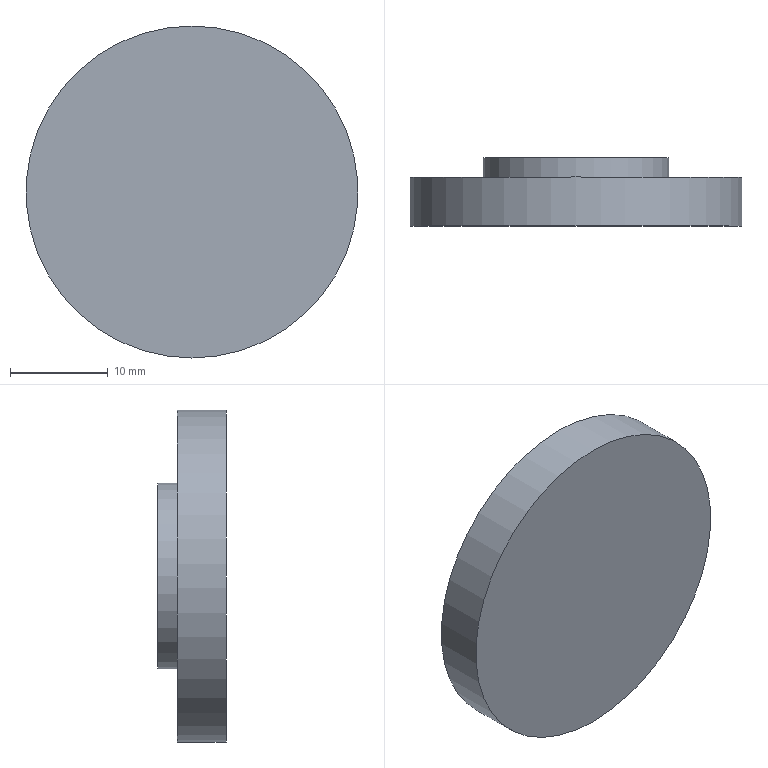Part | STEP file | zhoutao_φ16 | 1 solid | 7 faces | box 34 x 7 x 34 mm | volume 4705 mm3 | plane 4 | cylinder 3 | commonest cylinder face diameters 16 x1 19 x1 34 x1
STEP:
#1=CARTESIAN_POINT('',(0.,0.,0.));
#2=DIRECTION('',(0.,0.,1.));
#3=DIRECTION('',(1.,0.,0.));
#4=AXIS2_PLACEMENT_3D('',#1,#2,#3);
#5=CARTESIAN_POINT('',(0.,5.,17.));
#6=VERTEX_POINT('',#5);
#7=CARTESIAN_POINT('',(0.,5.,0.));
#8=DIRECTION('',(0.,1.,0.));
#9=DIRECTION('',(0.,0.,1.));
#10=AXIS2_PLACEMENT_3D('',#7,#8,#9);
#11=CIRCLE('',#10,17.);
#12=CARTESIAN_POINT('',(0.,5.,0.));
#13=DIRECTION('',(0.,-1.,0.));
#14=DIRECTION('',(0.,0.,-1.));
#15=AXIS2_PLACEMENT_3D('',#12,#13,#14);
#16=CYLINDRICAL_SURFACE('',#15,17.);
#17=CARTESIAN_POINT('',(9.425,0.));
#18=DIRECTION('',(-1.,0.));
#19=VECTOR('',#18,1.);
#20=LINE('',#17,#19);
#21=(GEOMETRIC_REPRESENTATION_CONTEXT(2)PARAMETRIC_REPRESENTATION_CONTEXT()REPRESENTATION_CONTEXT('',''));
#22=DEFINITIONAL_REPRESENTATION('',(#20),#21);
#23=PCURVE('',#16,#22);
#24=CARTESIAN_POINT('',(0.,5.,0.));
#25=DIRECTION('',(0.,1.,0.));
#26=DIRECTION('',(0.,0.,1.));
#27=AXIS2_PLACEMENT_3D('',#24,#25,#26);
#28=PLANE('',#27);
#29=CARTESIAN_POINT('',(0.,0.));
#30=DIRECTION('',(1.,0.));
#31=AXIS2_PLACEMENT_2D('',#29,#30);
#32=CIRCLE('',#31,17.);
#33=(GEOMETRIC_REPRESENTATION_CONTEXT(2)PARAMETRIC_REPRESENTATION_CONTEXT()REPRESENTATION_CONTEXT('',''));
#34=DEFINITIONAL_REPRESENTATION('',(#32),#33);
#35=PCURVE('',#28,#34);
#36=SURFACE_CURVE('',#11,(#23,#35),.PCURVE_S1.);
#37=EDGE_CURVE('',#6,#6,#36,.T.);
#38=ORIENTED_EDGE('',*,*,#37,.F.);
#39=CARTESIAN_POINT('',(0.,0.,17.));
#40=VERTEX_POINT('',#39);
#41=CARTESIAN_POINT('',(0.,5.,17.));
#42=CARTESIAN_POINT('',(0.,0.,17.));
#43=B_SPLINE_CURVE_WITH_KNOTS('',1,(#41,#42),.UNSPECIFIED.,.F.,.F.,(2,2),(0.,5.),.PIECEWISE_BEZIER_KNOTS.);
#44=CARTESIAN_POINT('',(9.425,0.));
#45=DIRECTION('',(0.,1.));
#46=VECTOR('',#45,1.);
#47=LINE('',#44,#46);
#48=(GEOMETRIC_REPRESENTATION_CONTEXT(2)PARAMETRIC_REPRESENTATION_CONTEXT()REPRESENTATION_CONTEXT('',''));
#49=DEFINITIONAL_REPRESENTATION('',(#47),#48);
#50=PCURVE('',#16,#49);
#51=CARTESIAN_POINT('',(3.142,0.));
#52=DIRECTION('',(0.,1.));
#53=VECTOR('',#52,1.);
#54=LINE('',#51,#53);
#55=(GEOMETRIC_REPRESENTATION_CONTEXT(2)PARAMETRIC_REPRESENTATION_CONTEXT()REPRESENTATION_CONTEXT('',''));
#56=DEFINITIONAL_REPRESENTATION('',(#54),#55);
#57=PCURVE('',#16,#56);
#58=SEAM_CURVE('',#43,(#50,#57),.PCURVE_S1.);
#59=EDGE_CURVE('',#6,#40,#58,.T.);
#60=ORIENTED_EDGE('',*,*,#59,.T.);
#61=CARTESIAN_POINT('',(0.,0.,0.));
#62=DIRECTION('',(0.,1.,0.));
#63=DIRECTION('',(0.,0.,1.));
#64=AXIS2_PLACEMENT_3D('',#61,#62,#63);
#65=CIRCLE('',#64,17.);
#66=CARTESIAN_POINT('',(9.425,5.));
#67=DIRECTION('',(-1.,0.));
#68=VECTOR('',#67,1.);
#69=LINE('',#66,#68);
#70=(GEOMETRIC_REPRESENTATION_CONTEXT(2)PARAMETRIC_REPRESENTATION_CONTEXT()REPRESENTATION_CONTEXT('',''));
#71=DEFINITIONAL_REPRESENTATION('',(#69),#70);
#72=PCURVE('',#16,#71);
#73=CARTESIAN_POINT('',(0.,0.,0.));
#74=DIRECTION('',(0.,1.,0.));
#75=DIRECTION('',(0.,0.,1.));
#76=AXIS2_PLACEMENT_3D('',#73,#74,#75);
#77=PLANE('',#76);
#78=CARTESIAN_POINT('',(0.,0.));
#79=DIRECTION('',(1.,0.));
#80=AXIS2_PLACEMENT_2D('',#78,#79);
#81=CIRCLE('',#80,17.);
#82=(GEOMETRIC_REPRESENTATION_CONTEXT(2)PARAMETRIC_REPRESENTATION_CONTEXT()REPRESENTATION_CONTEXT('',''));
#83=DEFINITIONAL_REPRESENTATION('',(#81),#82);
#84=PCURVE('',#77,#83);
#85=SURFACE_CURVE('',#65,(#72,#84),.PCURVE_S1.);
#86=EDGE_CURVE('',#40,#40,#85,.T.);
#87=ORIENTED_EDGE('',*,*,#86,.T.);
#88=ORIENTED_EDGE('',*,*,#59,.F.);
#89=EDGE_LOOP('',(#38,#60,#87,#88));
#90=FACE_BOUND('',#89,.T.);
#91=ADVANCED_FACE('',(#90),#16,.T.);
#92=CARTESIAN_POINT('',(0.,5.,9.5));
#93=VERTEX_POINT('',#92);
#94=CARTESIAN_POINT('',(0.,5.,0.));
#95=DIRECTION('',(0.,1.,0.));
#96=DIRECTION('',(0.,0.,1.));
#97=AXIS2_PLACEMENT_3D('',#94,#95,#96);
#98=CIRCLE('',#97,9.5);
#99=CARTESIAN_POINT('',(0.,0.));
#100=DIRECTION('',(1.,0.));
#101=AXIS2_PLACEMENT_2D('',#99,#100);
#102=CIRCLE('',#101,9.5);
#103=(GEOMETRIC_REPRESENTATION_CONTEXT(2)PARAMETRIC_REPRESENTATION_CONTEXT()REPRESENTATION_CONTEXT('',''));
#104=DEFINITIONAL_REPRESENTATION('',(#102),#103);
#105=PCURVE('',#28,#104);
#106=CARTESIAN_POINT('',(0.,7.,0.));
#107=DIRECTION('',(0.,-1.,0.));
#108=DIRECTION('',(0.,0.,-1.));
#109=AXIS2_PLACEMENT_3D('',#106,#107,#108);
#110=CYLINDRICAL_SURFACE('',#109,9.5);
#111=CARTESIAN_POINT('',(9.425,2.));
#112=DIRECTION('',(-1.,0.));
#113=VECTOR('',#112,1.);
#114=LINE('',#111,#113);
#115=(GEOMETRIC_REPRESENTATION_CONTEXT(2)PARAMETRIC_REPRESENTATION_CONTEXT()REPRESENTATION_CONTEXT('',''));
#116=DEFINITIONAL_REPRESENTATION('',(#114),#115);
#117=PCURVE('',#110,#116);
#118=SURFACE_CURVE('',#98,(#105,#117),.PCURVE_S1.);
#119=EDGE_CURVE('',#93,#93,#118,.T.);
#120=ORIENTED_EDGE('',*,*,#119,.F.);
#121=EDGE_LOOP('',(#120));
#122=FACE_BOUND('',#121,.T.);
#123=ORIENTED_EDGE('',*,*,#37,.T.);
#124=EDGE_LOOP('',(#123));
#125=FACE_BOUND('',#124,.T.);
#126=ADVANCED_FACE('',(#122,#125),#28,.T.);
#127=ORIENTED_EDGE('',*,*,#86,.F.);
#128=EDGE_LOOP('',(#127));
#129=FACE_BOUND('',#128,.T.);
#130=ADVANCED_FACE('',(#129),#77,.F.);
#131=CARTESIAN_POINT('',(0.,7.,9.5));
#132=VERTEX_POINT('',#131);
#133=CARTESIAN_POINT('',(0.,7.,0.));
#134=DIRECTION('',(0.,1.,0.));
#135=DIRECTION('',(0.,0.,1.));
#136=AXIS2_PLACEMENT_3D('',#133,#134,#135);
#137=CIRCLE('',#136,9.5);
#138=CARTESIAN_POINT('',(0.,7.,0.));
#139=DIRECTION('',(0.,1.,0.));
#140=DIRECTION('',(0.,0.,1.));
#141=AXIS2_PLACEMENT_3D('',#138,#139,#140);
#142=PLANE('',#141);
#143=CARTESIAN_POINT('',(0.,0.));
#144=DIRECTION('',(1.,0.));
#145=AXIS2_PLACEMENT_2D('',#143,#144);
#146=CIRCLE('',#145,9.5);
#147=(GEOMETRIC_REPRESENTATION_CONTEXT(2)PARAMETRIC_REPRESENTATION_CONTEXT()REPRESENTATION_CONTEXT('',''));
#148=DEFINITIONAL_REPRESENTATION('',(#146),#147);
#149=PCURVE('',#142,#148);
#150=CARTESIAN_POINT('',(9.425,0.));
#151=DIRECTION('',(-1.,0.));
#152=VECTOR('',#151,1.);
#153=LINE('',#150,#152);
#154=(GEOMETRIC_REPRESENTATION_CONTEXT(2)PARAMETRIC_REPRESENTATION_CONTEXT()REPRESENTATION_CONTEXT('',''));
#155=DEFINITIONAL_REPRESENTATION('',(#153),#154);
#156=PCURVE('',#110,#155);
#157=SURFACE_CURVE('',#137,(#149,#156),.PCURVE_S1.);
#158=EDGE_CURVE('',#132,#132,#157,.T.);
#159=ORIENTED_EDGE('',*,*,#158,.T.);
#160=EDGE_LOOP('',(#159));
#161=FACE_BOUND('',#160,.T.);
#162=CARTESIAN_POINT('',(0.,7.,8.));
#163=VERTEX_POINT('',#162);
#164=CARTESIAN_POINT('',(0.,7.,0.));
#165=DIRECTION('',(0.,1.,0.));
#166=DIRECTION('',(0.,0.,1.));
#167=AXIS2_PLACEMENT_3D('',#164,#165,#166);
#168=CIRCLE('',#167,8.);
#169=CARTESIAN_POINT('',(0.,0.));
#170=DIRECTION('',(1.,0.));
#171=AXIS2_PLACEMENT_2D('',#169,#170);
#172=CIRCLE('',#171,8.);
#173=(GEOMETRIC_REPRESENTATION_CONTEXT(2)PARAMETRIC_REPRESENTATION_CONTEXT()REPRESENTATION_CONTEXT('',''));
#174=DEFINITIONAL_REPRESENTATION('',(#172),#173);
#175=PCURVE('',#142,#174);
#176=CARTESIAN_POINT('',(0.,7.,0.));
#177=DIRECTION('',(0.,-1.,0.));
#178=DIRECTION('',(0.,0.,-1.));
#179=AXIS2_PLACEMENT_3D('',#176,#177,#178);
#180=CYLINDRICAL_SURFACE('',#179,8.);
#181=CARTESIAN_POINT('',(9.425,0.));
#182=DIRECTION('',(-1.,0.));
#183=VECTOR('',#182,1.);
#184=LINE('',#181,#183);
#185=(GEOMETRIC_REPRESENTATION_CONTEXT(2)PARAMETRIC_REPRESENTATION_CONTEXT()REPRESENTATION_CONTEXT('',''));
#186=DEFINITIONAL_REPRESENTATION('',(#184),#185);
#187=PCURVE('',#180,#186);
#188=SURFACE_CURVE('',#168,(#175,#187),.PCURVE_S1.);
#189=EDGE_CURVE('',#163,#163,#188,.T.);
#190=ORIENTED_EDGE('',*,*,#189,.F.);
#191=EDGE_LOOP('',(#190));
#192=FACE_BOUND('',#191,.T.);
#193=ADVANCED_FACE('',(#161,#192),#142,.T.);
#194=ORIENTED_EDGE('',*,*,#158,.F.);
#195=CARTESIAN_POINT('',(0.,7.,9.5));
#196=CARTESIAN_POINT('',(0.,5.,9.5));
#197=B_SPLINE_CURVE_WITH_KNOTS('',1,(#195,#196),.UNSPECIFIED.,.F.,.F.,(2,2),(0.,2.),.PIECEWISE_BEZIER_KNOTS.);
#198=CARTESIAN_POINT('',(9.425,0.));
#199=DIRECTION('',(0.,1.));
#200=VECTOR('',#199,1.);
#201=LINE('',#198,#200);
#202=(GEOMETRIC_REPRESENTATION_CONTEXT(2)PARAMETRIC_REPRESENTATION_CONTEXT()REPRESENTATION_CONTEXT('',''));
#203=DEFINITIONAL_REPRESENTATION('',(#201),#202);
#204=PCURVE('',#110,#203);
#205=CARTESIAN_POINT('',(3.142,0.));
#206=DIRECTION('',(0.,1.));
#207=VECTOR('',#206,1.);
#208=LINE('',#205,#207);
#209=(GEOMETRIC_REPRESENTATION_CONTEXT(2)PARAMETRIC_REPRESENTATION_CONTEXT()REPRESENTATION_CONTEXT('',''));
#210=DEFINITIONAL_REPRESENTATION('',(#208),#209);
#211=PCURVE('',#110,#210);
#212=SEAM_CURVE('',#197,(#204,#211),.PCURVE_S1.);
#213=EDGE_CURVE('',#132,#93,#212,.T.);
#214=ORIENTED_EDGE('',*,*,#213,.T.);
#215=ORIENTED_EDGE('',*,*,#119,.T.);
#216=ORIENTED_EDGE('',*,*,#213,.F.);
#217=EDGE_LOOP('',(#194,#214,#215,#216));
#218=FACE_BOUND('',#217,.T.);
#219=ADVANCED_FACE('',(#218),#110,.T.);
#220=ORIENTED_EDGE('',*,*,#189,.F.);
#221=CARTESIAN_POINT('',(0.,5.,8.));
#222=VERTEX_POINT('',#221);
#223=CARTESIAN_POINT('',(0.,7.,8.));
#224=CARTESIAN_POINT('',(0.,5.,8.));
#225=B_SPLINE_CURVE_WITH_KNOTS('',1,(#223,#224),.UNSPECIFIED.,.F.,.F.,(2,2),(0.,2.),.PIECEWISE_BEZIER_KNOTS.);
#226=CARTESIAN_POINT('',(9.425,0.));
#227=DIRECTION('',(0.,1.));
#228=VECTOR('',#227,1.);
#229=LINE('',#226,#228);
#230=(GEOMETRIC_REPRESENTATION_CONTEXT(2)PARAMETRIC_REPRESENTATION_CONTEXT()REPRESENTATION_CONTEXT('',''));
#231=DEFINITIONAL_REPRESENTATION('',(#229),#230);
#232=PCURVE('',#180,#231);
#233=CARTESIAN_POINT('',(3.142,0.));
#234=DIRECTION('',(0.,1.));
#235=VECTOR('',#234,1.);
#236=LINE('',#233,#235);
#237=(GEOMETRIC_REPRESENTATION_CONTEXT(2)PARAMETRIC_REPRESENTATION_CONTEXT()REPRESENTATION_CONTEXT('',''));
#238=DEFINITIONAL_REPRESENTATION('',(#236),#237);
#239=PCURVE('',#180,#238);
#240=SEAM_CURVE('',#225,(#232,#239),.PCURVE_S1.);
#241=EDGE_CURVE('',#163,#222,#240,.T.);
#242=ORIENTED_EDGE('',*,*,#241,.T.);
#243=CARTESIAN_POINT('',(0.,5.,0.));
#244=DIRECTION('',(0.,-1.,0.));
#245=DIRECTION('',(0.,0.,1.));
#246=AXIS2_PLACEMENT_3D('',#243,#244,#245);
#247=CIRCLE('',#246,8.);
#248=CARTESIAN_POINT('',(3.142,2.));
#249=DIRECTION('',(1.,0.));
#250=VECTOR('',#249,1.);
#251=LINE('',#248,#250);
#252=(GEOMETRIC_REPRESENTATION_CONTEXT(2)PARAMETRIC_REPRESENTATION_CONTEXT()REPRESENTATION_CONTEXT('',''));
#253=DEFINITIONAL_REPRESENTATION('',(#251),#252);
#254=PCURVE('',#180,#253);
#255=CARTESIAN_POINT('',(0.,5.,0.));
#256=DIRECTION('',(0.,1.,0.));
#257=DIRECTION('',(0.,0.,1.));
#258=AXIS2_PLACEMENT_3D('',#255,#256,#257);
#259=PLANE('',#258);
#260=CARTESIAN_POINT('',(8.,0.));
#261=CARTESIAN_POINT('',(8.,-13.856));
#262=CARTESIAN_POINT('',(-4.,-6.928));
#263=CARTESIAN_POINT('',(-16.,0.));
#264=CARTESIAN_POINT('',(-4.,6.928));
#265=CARTESIAN_POINT('',(8.,13.856));
#266=CARTESIAN_POINT('',(8.,0.));
#267=(BOUNDED_CURVE()B_SPLINE_CURVE(2,(#260,#261,#262,#263,#264,#265,#266),.UNSPECIFIED.,.T.,.F.)B_SPLINE_CURVE_WITH_KNOTS((1,2,2,2,2,1),(-2.094,0.,2.094,4.189,6.283,8.378),.UNSPECIFIED.)CURVE()GEOMETRIC_REPRESENTATION_ITEM()RATIONAL_B_SPLINE_CURVE((1.,0.5,1.,0.5,1.,0.5,1.))REPRESENTATION_ITEM(''));
#268=(GEOMETRIC_REPRESENTATION_CONTEXT(2)PARAMETRIC_REPRESENTATION_CONTEXT()REPRESENTATION_CONTEXT('',''));
#269=DEFINITIONAL_REPRESENTATION('',(#267),#268);
#270=PCURVE('',#259,#269);
#271=SURFACE_CURVE('',#247,(#254,#270),.PCURVE_S1.);
#272=EDGE_CURVE('',#222,#222,#271,.T.);
#273=ORIENTED_EDGE('',*,*,#272,.F.);
#274=ORIENTED_EDGE('',*,*,#241,.F.);
#275=EDGE_LOOP('',(#220,#242,#273,#274));
#276=FACE_BOUND('',#275,.F.);
#277=ADVANCED_FACE('',(#276),#180,.F.);
#278=ORIENTED_EDGE('',*,*,#272,.F.);
#279=EDGE_LOOP('',(#278));
#280=FACE_BOUND('',#279,.T.);
#281=ADVANCED_FACE('',(#280),#259,.T.);
#282=CLOSED_SHELL('',(#91,#126,#130,#193,#219,#277,#281));
#283=MANIFOLD_SOLID_BREP('',#282);
#284=(LENGTH_UNIT()NAMED_UNIT(*)SI_UNIT(.MILLI.,.METRE.));
#285=UNCERTAINTY_MEASURE_WITH_UNIT(LENGTH_MEASURE(0.00001),#284,'','');
#286=(NAMED_UNIT(*)PLANE_ANGLE_UNIT()SI_UNIT($,.RADIAN.));
#287=(NAMED_UNIT(*)SI_UNIT($,.STERADIAN.)SOLID_ANGLE_UNIT());
#288=(GEOMETRIC_REPRESENTATION_CONTEXT(3)GLOBAL_UNCERTAINTY_ASSIGNED_CONTEXT((#285))GLOBAL_UNIT_ASSIGNED_CONTEXT((#284,#286,#287))REPRESENTATION_CONTEXT('',''));
#289=ADVANCED_BREP_SHAPE_REPRESENTATION('',(#4,#283),#288);